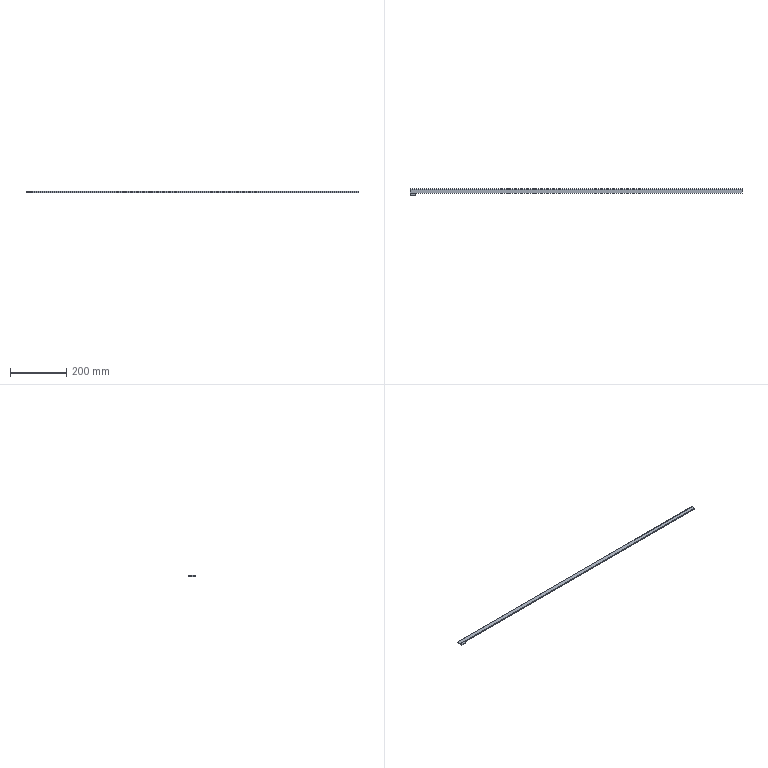Part | SolidWorks | features Extrusion 1, Fillet 1, ICE 1 | 2 solids | 13 faces | box 1185 x 24 x 4 mm | volume 74446 mm3 | plane 11 | cylinder 2 | commonest cylinder face diameters 4 x2
STEP:
#1=CARTESIAN_POINT('',(-592.5,14.,2.));
#2=VERTEX_POINT('',#1);
#3=CARTESIAN_POINT('',(-592.5,16.,0.));
#4=VERTEX_POINT('',#3);
#5=CARTESIAN_POINT('',(-592.5,14.,0.));
#6=DIRECTION('',(-1.,0.,0.));
#7=DIRECTION('',(0.,0.,-1.));
#8=AXIS2_PLACEMENT_3D('',#5,#6,#7);
#9=CIRCLE('',#8,2.);
#10=EDGE_CURVE('',#2,#4,#9,.T.);
#11=ORIENTED_EDGE('',*,*,#10,.T.);
#12=CARTESIAN_POINT('',(-592.5,14.,-2.));
#13=VERTEX_POINT('',#12);
#14=CARTESIAN_POINT('',(-592.5,14.,0.));
#15=DIRECTION('',(-1.,0.,0.));
#16=DIRECTION('',(0.,0.,-1.));
#17=AXIS2_PLACEMENT_3D('',#14,#15,#16);
#18=CIRCLE('',#17,2.);
#19=EDGE_CURVE('',#4,#13,#18,.T.);
#20=ORIENTED_EDGE('',*,*,#19,.T.);
#21=CARTESIAN_POINT('',(-592.5,0.,-2.));
#22=VERTEX_POINT('',#21);
#23=CARTESIAN_POINT('',(-592.5,16.,-2.));
#24=DIRECTION('',(0.,-1.,0.));
#25=VECTOR('',#24,1000.);
#26=LINE('',#23,#25);
#27=EDGE_CURVE('',#13,#22,#26,.T.);
#28=ORIENTED_EDGE('',*,*,#27,.T.);
#29=CARTESIAN_POINT('',(-592.5,0.,2.));
#30=VERTEX_POINT('',#29);
#31=CARTESIAN_POINT('',(-592.5,0.,2.));
#32=DIRECTION('',(0.,0.,1.));
#33=VECTOR('',#32,1000.);
#34=LINE('',#31,#33);
#35=EDGE_CURVE('',#22,#30,#34,.T.);
#36=ORIENTED_EDGE('',*,*,#35,.T.);
#37=CARTESIAN_POINT('',(-592.5,16.,2.));
#38=DIRECTION('',(0.,-1.,0.));
#39=VECTOR('',#38,1000.);
#40=LINE('',#37,#39);
#41=EDGE_CURVE('',#2,#30,#40,.T.);
#42=ORIENTED_EDGE('',*,*,#41,.F.);
#43=EDGE_LOOP('',(#11,#20,#28,#36,#42));
#44=FACE_OUTER_BOUND('',#43,.T.);
#45=CARTESIAN_POINT('',(-592.5,16.,2.));
#46=DIRECTION('',(1.,0.,0.));
#47=DIRECTION('',(0.,0.,-1.));
#48=AXIS2_PLACEMENT_3D('',#45,#46,#47);
#49=PLANE('',#48);
#50=ADVANCED_FACE('',(#44),#49,.F.);
#51=CARTESIAN_POINT('',(592.5,14.,2.));
#52=VERTEX_POINT('',#51);
#53=CARTESIAN_POINT('',(592.5,0.,2.));
#54=VERTEX_POINT('',#53);
#55=CARTESIAN_POINT('',(592.5,16.,2.));
#56=DIRECTION('',(0.,-1.,0.));
#57=VECTOR('',#56,1000.);
#58=LINE('',#55,#57);
#59=EDGE_CURVE('',#52,#54,#58,.T.);
#60=ORIENTED_EDGE('',*,*,#59,.F.);
#61=CARTESIAN_POINT('',(-592.5,14.,2.));
#62=DIRECTION('',(-1.,0.,0.));
#63=VECTOR('',#62,1000.);
#64=LINE('',#61,#63);
#65=EDGE_CURVE('',#52,#2,#64,.T.);
#66=ORIENTED_EDGE('',*,*,#65,.T.);
#67=ORIENTED_EDGE('',*,*,#41,.T.);
#68=CARTESIAN_POINT('',(592.5,0.,2.));
#69=DIRECTION('',(1.,0.,0.));
#70=VECTOR('',#69,1000.);
#71=LINE('',#68,#70);
#72=EDGE_CURVE('',#30,#54,#71,.T.);
#73=ORIENTED_EDGE('',*,*,#72,.T.);
#74=EDGE_LOOP('',(#60,#66,#67,#73));
#75=FACE_OUTER_BOUND('',#74,.T.);
#76=CARTESIAN_POINT('',(592.5,16.,2.));
#77=DIRECTION('',(0.,0.,-1.));
#78=DIRECTION('',(-1.,0.,0.));
#79=AXIS2_PLACEMENT_3D('',#76,#77,#78);
#80=PLANE('',#79);
#81=ADVANCED_FACE('',(#75),#80,.F.);
#82=CARTESIAN_POINT('',(592.5,14.,-2.));
#83=VERTEX_POINT('',#82);
#84=CARTESIAN_POINT('',(592.5,0.,-2.));
#85=VERTEX_POINT('',#84);
#86=CARTESIAN_POINT('',(592.5,16.,-2.));
#87=DIRECTION('',(0.,-1.,0.));
#88=VECTOR('',#87,1000.);
#89=LINE('',#86,#88);
#90=EDGE_CURVE('',#83,#85,#89,.T.);
#91=ORIENTED_EDGE('',*,*,#90,.F.);
#92=CARTESIAN_POINT('',(592.5,16.,0.));
#93=VERTEX_POINT('',#92);
#94=CARTESIAN_POINT('',(592.5,14.,0.));
#95=DIRECTION('',(1.,0.,0.));
#96=DIRECTION('',(0.,0.,1.));
#97=AXIS2_PLACEMENT_3D('',#94,#95,#96);
#98=CIRCLE('',#97,2.);
#99=EDGE_CURVE('',#83,#93,#98,.T.);
#100=ORIENTED_EDGE('',*,*,#99,.T.);
#101=CARTESIAN_POINT('',(592.5,14.,0.));
#102=DIRECTION('',(1.,0.,0.));
#103=DIRECTION('',(0.,0.,1.));
#104=AXIS2_PLACEMENT_3D('',#101,#102,#103);
#105=CIRCLE('',#104,2.);
#106=EDGE_CURVE('',#93,#52,#105,.T.);
#107=ORIENTED_EDGE('',*,*,#106,.T.);
#108=ORIENTED_EDGE('',*,*,#59,.T.);
#109=CARTESIAN_POINT('',(592.5,0.,2.));
#110=DIRECTION('',(0.,0.,-1.));
#111=VECTOR('',#110,1000.);
#112=LINE('',#109,#111);
#113=EDGE_CURVE('',#54,#85,#112,.T.);
#114=ORIENTED_EDGE('',*,*,#113,.T.);
#115=EDGE_LOOP('',(#91,#100,#107,#108,#114));
#116=FACE_OUTER_BOUND('',#115,.T.);
#117=CARTESIAN_POINT('',(592.5,16.,2.));
#118=DIRECTION('',(-1.,0.,0.));
#119=DIRECTION('',(0.,0.,1.));
#120=AXIS2_PLACEMENT_3D('',#117,#118,#119);
#121=PLANE('',#120);
#122=ADVANCED_FACE('',(#116),#121,.F.);
#123=ORIENTED_EDGE('',*,*,#27,.F.);
#124=CARTESIAN_POINT('',(592.5,14.,-2.));
#125=DIRECTION('',(1.,0.,0.));
#126=VECTOR('',#125,1000.);
#127=LINE('',#124,#126);
#128=EDGE_CURVE('',#13,#83,#127,.T.);
#129=ORIENTED_EDGE('',*,*,#128,.T.);
#130=ORIENTED_EDGE('',*,*,#90,.T.);
#131=CARTESIAN_POINT('',(592.5,0.,-2.));
#132=DIRECTION('',(-1.,0.,0.));
#133=VECTOR('',#132,1000.);
#134=LINE('',#131,#133);
#135=EDGE_CURVE('',#85,#22,#134,.T.);
#136=ORIENTED_EDGE('',*,*,#135,.T.);
#137=EDGE_LOOP('',(#123,#129,#130,#136));
#138=FACE_OUTER_BOUND('',#137,.T.);
#139=CARTESIAN_POINT('',(592.5,16.,-2.));
#140=DIRECTION('',(0.,0.,1.));
#141=DIRECTION('',(1.,0.,0.));
#142=AXIS2_PLACEMENT_3D('',#139,#140,#141);
#143=PLANE('',#142);
#144=ADVANCED_FACE('',(#138),#143,.F.);
#145=ORIENTED_EDGE('',*,*,#35,.F.);
#146=ORIENTED_EDGE('',*,*,#135,.F.);
#147=ORIENTED_EDGE('',*,*,#113,.F.);
#148=ORIENTED_EDGE('',*,*,#72,.F.);
#149=EDGE_LOOP('',(#145,#146,#147,#148));
#150=FACE_OUTER_BOUND('',#149,.T.);
#151=CARTESIAN_POINT('',(0.,0.,0.));
#152=DIRECTION('',(0.,1.,0.));
#153=DIRECTION('',(0.,0.,1.));
#154=AXIS2_PLACEMENT_3D('',#151,#152,#153);
#155=PLANE('',#154);
#156=ADVANCED_FACE('',(#150),#155,.F.);
#157=ORIENTED_EDGE('',*,*,#65,.F.);
#158=ORIENTED_EDGE('',*,*,#106,.F.);
#159=CARTESIAN_POINT('',(592.5,16.,0.));
#160=DIRECTION('',(1.,0.,0.));
#161=VECTOR('',#160,1000.);
#162=LINE('',#159,#161);
#163=EDGE_CURVE('',#4,#93,#162,.T.);
#164=ORIENTED_EDGE('',*,*,#163,.F.);
#165=ORIENTED_EDGE('',*,*,#10,.F.);
#166=EDGE_LOOP('',(#157,#158,#164,#165));
#167=FACE_OUTER_BOUND('',#166,.T.);
#168=CARTESIAN_POINT('',(0.,14.,0.));
#169=DIRECTION('',(-1.,0.,0.));
#170=DIRECTION('',(0.,0.,1.));
#171=AXIS2_PLACEMENT_3D('',#168,#169,#170);
#172=CYLINDRICAL_SURFACE('',#171,2.);
#173=ADVANCED_FACE('',(#167),#172,.T.);
#174=ORIENTED_EDGE('',*,*,#99,.F.);
#175=ORIENTED_EDGE('',*,*,#128,.F.);
#176=ORIENTED_EDGE('',*,*,#19,.F.);
#177=ORIENTED_EDGE('',*,*,#163,.T.);
#178=EDGE_LOOP('',(#174,#175,#176,#177));
#179=FACE_OUTER_BOUND('',#178,.T.);
#180=CARTESIAN_POINT('',(0.,14.,0.));
#181=DIRECTION('',(1.,0.,0.));
#182=DIRECTION('',(0.,0.,-1.));
#183=AXIS2_PLACEMENT_3D('',#180,#181,#182);
#184=CYLINDRICAL_SURFACE('',#183,2.);
#185=ADVANCED_FACE('',(#179),#184,.T.);
#186=CLOSED_SHELL('',(#50,#81,#122,#144,#156,#173,#185));
#187=MANIFOLD_SOLID_BREP('',#186);
#188=CARTESIAN_POINT('',(-572.5,0.,-2.));
#189=VERTEX_POINT('',#188);
#190=CARTESIAN_POINT('',(-572.5,0.,2.));
#191=VERTEX_POINT('',#190);
#192=CARTESIAN_POINT('',(-572.5,0.,2.));
#193=DIRECTION('',(0.,0.,1.));
#194=VECTOR('',#193,1000.);
#195=LINE('',#192,#194);
#196=EDGE_CURVE('',#189,#191,#195,.T.);
#197=ORIENTED_EDGE('',*,*,#196,.T.);
#198=CARTESIAN_POINT('',(-572.5,-8.,2.));
#199=VERTEX_POINT('',#198);
#200=CARTESIAN_POINT('',(-572.5,-8.,2.));
#201=DIRECTION('',(0.,1.,0.));
#202=VECTOR('',#201,1000.);
#203=LINE('',#200,#202);
#204=EDGE_CURVE('',#199,#191,#203,.T.);
#205=ORIENTED_EDGE('',*,*,#204,.F.);
#206=CARTESIAN_POINT('',(-572.5,-8.,-2.));
#207=VERTEX_POINT('',#206);
#208=CARTESIAN_POINT('',(-572.5,-8.,2.));
#209=DIRECTION('',(0.,0.,1.));
#210=VECTOR('',#209,1000.);
#211=LINE('',#208,#210);
#212=EDGE_CURVE('',#207,#199,#211,.T.);
#213=ORIENTED_EDGE('',*,*,#212,.F.);
#214=CARTESIAN_POINT('',(-572.5,-8.,-2.));
#215=DIRECTION('',(0.,1.,0.));
#216=VECTOR('',#215,1000.);
#217=LINE('',#214,#216);
#218=EDGE_CURVE('',#207,#189,#217,.T.);
#219=ORIENTED_EDGE('',*,*,#218,.T.);
#220=EDGE_LOOP('',(#197,#205,#213,#219));
#221=FACE_OUTER_BOUND('',#220,.T.);
#222=CARTESIAN_POINT('',(-572.5,-8.,2.));
#223=DIRECTION('',(-1.,0.,0.));
#224=DIRECTION('',(0.,0.,1.));
#225=AXIS2_PLACEMENT_3D('',#222,#223,#224);
#226=PLANE('',#225);
#227=ADVANCED_FACE('',(#221),#226,.F.);
#228=CARTESIAN_POINT('',(-592.5,0.,2.));
#229=VERTEX_POINT('',#228);
#230=CARTESIAN_POINT('',(-572.5,0.,2.));
#231=DIRECTION('',(-1.,0.,0.));
#232=VECTOR('',#231,1000.);
#233=LINE('',#230,#232);
#234=EDGE_CURVE('',#191,#229,#233,.T.);
#235=ORIENTED_EDGE('',*,*,#234,.T.);
#236=CARTESIAN_POINT('',(-592.5,-8.,2.));
#237=VERTEX_POINT('',#236);
#238=CARTESIAN_POINT('',(-592.5,-8.,2.));
#239=DIRECTION('',(0.,1.,0.));
#240=VECTOR('',#239,1000.);
#241=LINE('',#238,#240);
#242=EDGE_CURVE('',#237,#229,#241,.T.);
#243=ORIENTED_EDGE('',*,*,#242,.F.);
#244=CARTESIAN_POINT('',(-572.5,-8.,2.));
#245=DIRECTION('',(-1.,0.,0.));
#246=VECTOR('',#245,1000.);
#247=LINE('',#244,#246);
#248=EDGE_CURVE('',#199,#237,#247,.T.);
#249=ORIENTED_EDGE('',*,*,#248,.F.);
#250=ORIENTED_EDGE('',*,*,#204,.T.);
#251=EDGE_LOOP('',(#235,#243,#249,#250));
#252=FACE_OUTER_BOUND('',#251,.T.);
#253=CARTESIAN_POINT('',(-572.5,-8.,2.));
#254=DIRECTION('',(0.,0.,-1.));
#255=DIRECTION('',(-1.,0.,0.));
#256=AXIS2_PLACEMENT_3D('',#253,#254,#255);
#257=PLANE('',#256);
#258=ADVANCED_FACE('',(#252),#257,.F.);
#259=CARTESIAN_POINT('',(-592.5,0.,-2.));
#260=VERTEX_POINT('',#259);
#261=CARTESIAN_POINT('',(-592.5,0.,2.));
#262=DIRECTION('',(0.,0.,-1.));
#263=VECTOR('',#262,1000.);
#264=LINE('',#261,#263);
#265=EDGE_CURVE('',#229,#260,#264,.T.);
#266=ORIENTED_EDGE('',*,*,#265,.T.);
#267=CARTESIAN_POINT('',(-592.5,-8.,-2.));
#268=VERTEX_POINT('',#267);
#269=CARTESIAN_POINT('',(-592.5,-8.,-2.));
#270=DIRECTION('',(0.,1.,0.));
#271=VECTOR('',#270,1000.);
#272=LINE('',#269,#271);
#273=EDGE_CURVE('',#268,#260,#272,.T.);
#274=ORIENTED_EDGE('',*,*,#273,.F.);
#275=CARTESIAN_POINT('',(-592.5,-8.,2.));
#276=DIRECTION('',(0.,0.,-1.));
#277=VECTOR('',#276,1000.);
#278=LINE('',#275,#277);
#279=EDGE_CURVE('',#237,#268,#278,.T.);
#280=ORIENTED_EDGE('',*,*,#279,.F.);
#281=ORIENTED_EDGE('',*,*,#242,.T.);
#282=EDGE_LOOP('',(#266,#274,#280,#281));
#283=FACE_OUTER_BOUND('',#282,.T.);
#284=CARTESIAN_POINT('',(-592.5,-8.,2.));
#285=DIRECTION('',(1.,0.,0.));
#286=DIRECTION('',(0.,0.,-1.));
#287=AXIS2_PLACEMENT_3D('',#284,#285,#286);
#288=PLANE('',#287);
#289=ADVANCED_FACE('',(#283),#288,.F.);
#290=CARTESIAN_POINT('',(-572.5,0.,-2.));
#291=DIRECTION('',(1.,0.,0.));
#292=VECTOR('',#291,1000.);
#293=LINE('',#290,#292);
#294=EDGE_CURVE('',#260,#189,#293,.T.);
#295=ORIENTED_EDGE('',*,*,#294,.T.);
#296=ORIENTED_EDGE('',*,*,#218,.F.);
#297=CARTESIAN_POINT('',(-572.5,-8.,-2.));
#298=DIRECTION('',(1.,0.,0.));
#299=VECTOR('',#298,1000.);
#300=LINE('',#297,#299);
#301=EDGE_CURVE('',#268,#207,#300,.T.);
#302=ORIENTED_EDGE('',*,*,#301,.F.);
#303=ORIENTED_EDGE('',*,*,#273,.T.);
#304=EDGE_LOOP('',(#295,#296,#302,#303));
#305=FACE_OUTER_BOUND('',#304,.T.);
#306=CARTESIAN_POINT('',(-572.5,-8.,-2.));
#307=DIRECTION('',(0.,0.,1.));
#308=DIRECTION('',(1.,0.,0.));
#309=AXIS2_PLACEMENT_3D('',#306,#307,#308);
#310=PLANE('',#309);
#311=ADVANCED_FACE('',(#305),#310,.F.);
#312=ORIENTED_EDGE('',*,*,#212,.T.);
#313=ORIENTED_EDGE('',*,*,#248,.T.);
#314=ORIENTED_EDGE('',*,*,#279,.T.);
#315=ORIENTED_EDGE('',*,*,#301,.T.);
#316=EDGE_LOOP('',(#312,#313,#314,#315));
#317=FACE_OUTER_BOUND('',#316,.T.);
#318=CARTESIAN_POINT('',(0.,-8.,0.));
#319=DIRECTION('',(0.,1.,0.));
#320=DIRECTION('',(0.,0.,1.));
#321=AXIS2_PLACEMENT_3D('',#318,#319,#320);
#322=PLANE('',#321);
#323=ADVANCED_FACE('',(#317),#322,.F.);
#324=ORIENTED_EDGE('',*,*,#196,.F.);
#325=ORIENTED_EDGE('',*,*,#294,.F.);
#326=ORIENTED_EDGE('',*,*,#265,.F.);
#327=ORIENTED_EDGE('',*,*,#234,.F.);
#328=EDGE_LOOP('',(#324,#325,#326,#327));
#329=FACE_OUTER_BOUND('',#328,.T.);
#330=CARTESIAN_POINT('',(0.,0.,0.));
#331=DIRECTION('',(0.,1.,0.));
#332=DIRECTION('',(0.,0.,1.));
#333=AXIS2_PLACEMENT_3D('',#330,#331,#332);
#334=PLANE('',#333);
#335=ADVANCED_FACE('',(#329),#334,.T.);
#336=CLOSED_SHELL('',(#227,#258,#289,#311,#323,#335));
#337=MANIFOLD_SOLID_BREP('',#336);
#338=CARTESIAN_POINT('',(0.,0.,0.));
#339=DIRECTION('',(0.,0.,1.));
#340=DIRECTION('',(1.,0.,0.));
#341=AXIS2_PLACEMENT_3D('',#338,#339,#340);
#342=(LENGTH_UNIT()NAMED_UNIT(*)SI_UNIT(.MILLI.,.METRE.));
#343=UNCERTAINTY_MEASURE_WITH_UNIT(LENGTH_MEASURE(0.00001),#342,'','');
#344=(NAMED_UNIT(*)PLANE_ANGLE_UNIT()SI_UNIT($,.RADIAN.));
#345=(NAMED_UNIT(*)SI_UNIT($,.STERADIAN.)SOLID_ANGLE_UNIT());
#346=(GEOMETRIC_REPRESENTATION_CONTEXT(3)GLOBAL_UNCERTAINTY_ASSIGNED_CONTEXT((#343))GLOBAL_UNIT_ASSIGNED_CONTEXT((#342,#344,#345))REPRESENTATION_CONTEXT('',''));
#347=ADVANCED_BREP_SHAPE_REPRESENTATION('',(#187,#337,#341),#346);